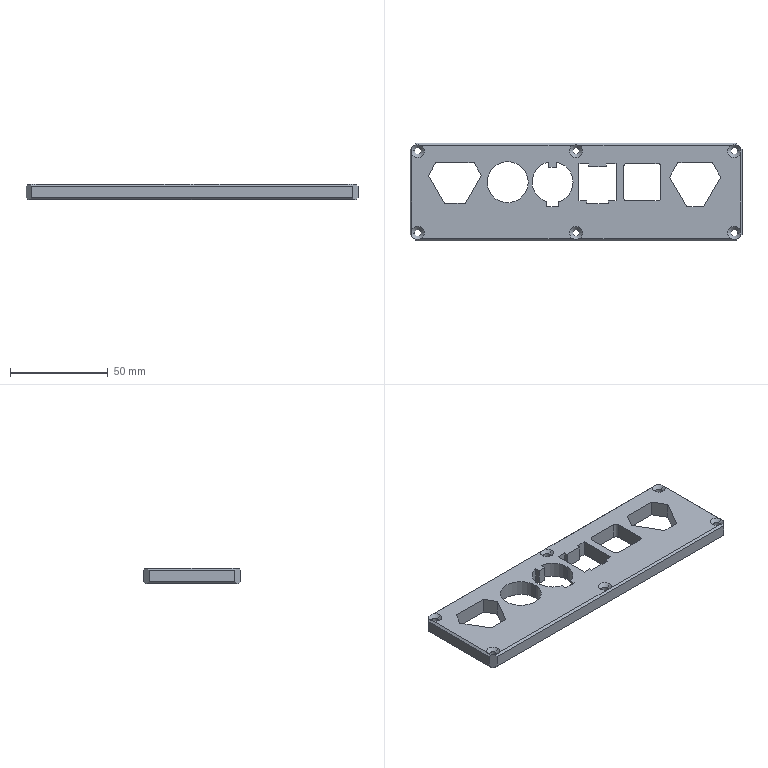Part | STEP file | Guard plate | 1 solid | 89 faces | box 170 x 50 x 8 mm | volume 48727 mm3 | plane 56 | cylinder 21 | cone 12 | commonest cylinder face diameters 3.4 x12 21 x5 3 x4